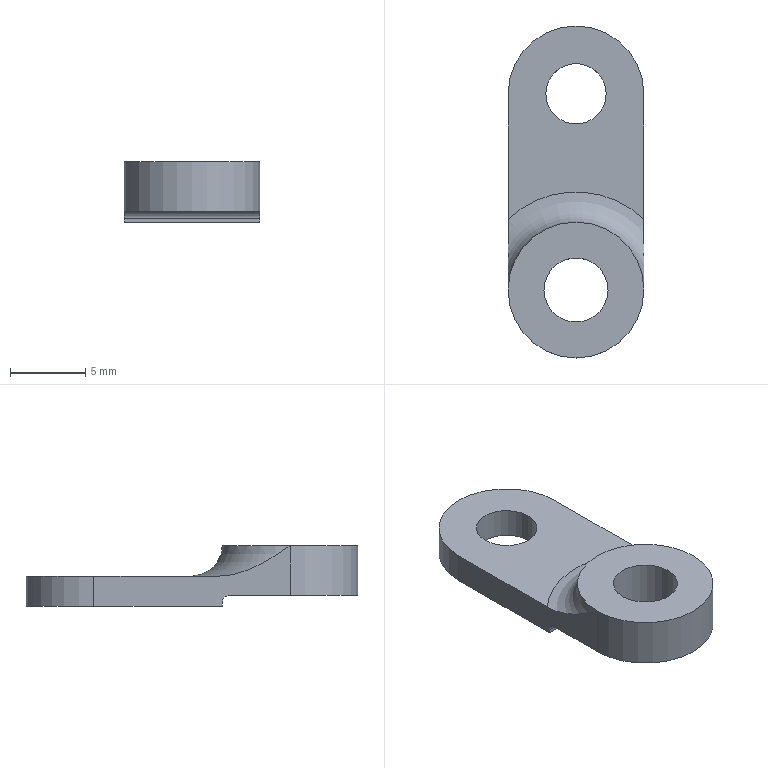Part | NX | 1 solid | 13 faces | box 9 x 22 x 4 mm | volume 375.215 mm3 | plane 7 | cylinder 5 | torus 1 | commonest cylinder face diameters 9 x2 1 x1 4 x1 4.25 x1
STEP:
#1=CARTESIAN_POINT('',(-4.5,-8.5,-1.78));
#2=VERTEX_POINT('',#1);
#3=CARTESIAN_POINT('',(-4.5,-8.5,-2.));
#4=VERTEX_POINT('',#3);
#5=CARTESIAN_POINT('',(-4.5,-8.5,-2.));
#6=DIRECTION('',(0.,0.,-1.));
#7=VECTOR('',#6,1000.);
#8=LINE('',#5,#7);
#9=EDGE_CURVE('',#2,#4,#8,.T.);
#10=ORIENTED_EDGE('',*,*,#9,.F.);
#11=CARTESIAN_POINT('',(-4.5,-9.,-1.28));
#12=VERTEX_POINT('',#11);
#13=CARTESIAN_POINT('',(-4.5,-9.,-1.78));
#14=DIRECTION('',(-1.,0.,0.));
#15=DIRECTION('',(0.,0.,1.));
#16=AXIS2_PLACEMENT_3D('',#13,#14,#15);
#17=CIRCLE('',#16,0.5);
#18=EDGE_CURVE('',#2,#12,#17,.F.);
#19=ORIENTED_EDGE('',*,*,#18,.T.);
#20=CARTESIAN_POINT('',(-4.5,-13.,-1.28));
#21=VERTEX_POINT('',#20);
#22=CARTESIAN_POINT('',(-4.5,0.,-1.28));
#23=DIRECTION('',(0.,1.,0.));
#24=VECTOR('',#23,1000.);
#25=LINE('',#22,#24);
#26=EDGE_CURVE('',#12,#21,#25,.F.);
#27=ORIENTED_EDGE('',*,*,#26,.T.);
#28=CARTESIAN_POINT('',(-4.5,-13.,2.));
#29=VERTEX_POINT('',#28);
#30=CARTESIAN_POINT('',(-4.5,-13.,-2.));
#31=DIRECTION('',(0.,0.,1.));
#32=VECTOR('',#31,1000.);
#33=LINE('',#30,#32);
#34=EDGE_CURVE('',#21,#29,#33,.T.);
#35=ORIENTED_EDGE('',*,*,#34,.T.);
#36=CARTESIAN_POINT('',(-4.5,-8.31,0.));
#37=VERTEX_POINT('',#36);
#38=CARTESIAN_POINT('',(-4.5,-8.31,0.));
#39=CARTESIAN_POINT('',(-4.5,-9.186,0.));
#40=CARTESIAN_POINT('',(-4.5,-10.86,0.5704));
#41=CARTESIAN_POINT('',(-4.5,-12.281,1.521));
#42=CARTESIAN_POINT('',(-4.5,-13.,2.));
#43=B_SPLINE_CURVE_WITH_KNOTS('',3,(#38,#39,#40,#41,#42),.UNSPECIFIED.,.F.,.F.,(4,1,4),(0.,0.002591,0.005182),.UNSPECIFIED.);
#44=EDGE_CURVE('',#29,#37,#43,.F.);
#45=ORIENTED_EDGE('',*,*,#44,.T.);
#46=CARTESIAN_POINT('',(-4.5,0.,0.));
#47=VERTEX_POINT('',#46);
#48=CARTESIAN_POINT('',(-4.5,0.,0.));
#49=DIRECTION('',(0.,-1.,0.));
#50=VECTOR('',#49,1000.);
#51=LINE('',#48,#50);
#52=EDGE_CURVE('',#47,#37,#51,.T.);
#53=ORIENTED_EDGE('',*,*,#52,.F.);
#54=CARTESIAN_POINT('',(-4.5,0.,-2.));
#55=VERTEX_POINT('',#54);
#56=CARTESIAN_POINT('',(-4.5,0.,-2.));
#57=DIRECTION('',(0.,0.,1.));
#58=VECTOR('',#57,1000.);
#59=LINE('',#56,#58);
#60=EDGE_CURVE('',#55,#47,#59,.T.);
#61=ORIENTED_EDGE('',*,*,#60,.F.);
#62=CARTESIAN_POINT('',(-4.5,0.,-2.));
#63=DIRECTION('',(0.,-1.,0.));
#64=VECTOR('',#63,1000.);
#65=LINE('',#62,#64);
#66=EDGE_CURVE('',#55,#4,#65,.T.);
#67=ORIENTED_EDGE('',*,*,#66,.T.);
#68=EDGE_LOOP('',(#10,#19,#27,#35,#45,#53,#61,#67));
#69=FACE_BOUND('',#68,.T.);
#70=CARTESIAN_POINT('',(-4.5,0.,-2.));
#71=DIRECTION('',(-1.,0.,0.));
#72=DIRECTION('',(0.,0.,1.));
#73=AXIS2_PLACEMENT_3D('',#70,#71,#72);
#74=PLANE('',#73);
#75=ADVANCED_FACE('',(#69),#74,.T.);
#76=ORIENTED_EDGE('',*,*,#60,.T.);
#77=CARTESIAN_POINT('',(4.5,0.,0.));
#78=VERTEX_POINT('',#77);
#79=CARTESIAN_POINT('',(0.,0.,0.));
#80=DIRECTION('',(0.,0.,1.));
#81=DIRECTION('',(1.,0.,0.));
#82=AXIS2_PLACEMENT_3D('',#79,#80,#81);
#83=CIRCLE('',#82,4.5);
#84=EDGE_CURVE('',#78,#47,#83,.T.);
#85=ORIENTED_EDGE('',*,*,#84,.F.);
#86=CARTESIAN_POINT('',(4.5,0.,-2.));
#87=VERTEX_POINT('',#86);
#88=CARTESIAN_POINT('',(4.5,0.,-2.));
#89=DIRECTION('',(0.,0.,1.));
#90=VECTOR('',#89,1000.);
#91=LINE('',#88,#90);
#92=EDGE_CURVE('',#87,#78,#91,.T.);
#93=ORIENTED_EDGE('',*,*,#92,.F.);
#94=CARTESIAN_POINT('',(0.,0.,-2.));
#95=DIRECTION('',(0.,0.,1.));
#96=DIRECTION('',(1.,0.,0.));
#97=AXIS2_PLACEMENT_3D('',#94,#95,#96);
#98=CIRCLE('',#97,4.5);
#99=EDGE_CURVE('',#87,#55,#98,.T.);
#100=ORIENTED_EDGE('',*,*,#99,.T.);
#101=EDGE_LOOP('',(#76,#85,#93,#100));
#102=FACE_BOUND('',#101,.T.);
#103=CARTESIAN_POINT('',(0.,0.,-2.));
#104=DIRECTION('',(0.,0.,1.));
#105=DIRECTION('',(1.,0.,0.));
#106=AXIS2_PLACEMENT_3D('',#103,#104,#105);
#107=CYLINDRICAL_SURFACE('',#106,4.5);
#108=ADVANCED_FACE('',(#102),#107,.T.);
#109=CARTESIAN_POINT('',(4.5,-13.,-1.28));
#110=VERTEX_POINT('',#109);
#111=CARTESIAN_POINT('',(4.5,-9.,-1.28));
#112=VERTEX_POINT('',#111);
#113=CARTESIAN_POINT('',(4.5,-13.,-1.28));
#114=DIRECTION('',(0.,-1.,0.));
#115=VECTOR('',#114,1000.);
#116=LINE('',#113,#115);
#117=EDGE_CURVE('',#110,#112,#116,.F.);
#118=ORIENTED_EDGE('',*,*,#117,.T.);
#119=CARTESIAN_POINT('',(4.5,-8.5,-1.78));
#120=VERTEX_POINT('',#119);
#121=CARTESIAN_POINT('',(4.5,-9.,-1.78));
#122=DIRECTION('',(1.,0.,0.));
#123=DIRECTION('',(0.,0.,-1.));
#124=AXIS2_PLACEMENT_3D('',#121,#122,#123);
#125=CIRCLE('',#124,0.5);
#126=EDGE_CURVE('',#112,#120,#125,.F.);
#127=ORIENTED_EDGE('',*,*,#126,.T.);
#128=CARTESIAN_POINT('',(4.5,-8.5,-2.));
#129=VERTEX_POINT('',#128);
#130=CARTESIAN_POINT('',(4.5,-8.5,-2.));
#131=DIRECTION('',(0.,0.,1.));
#132=VECTOR('',#131,1000.);
#133=LINE('',#130,#132);
#134=EDGE_CURVE('',#120,#129,#133,.F.);
#135=ORIENTED_EDGE('',*,*,#134,.T.);
#136=CARTESIAN_POINT('',(4.5,-13.,-2.));
#137=DIRECTION('',(0.,1.,0.));
#138=VECTOR('',#137,1000.);
#139=LINE('',#136,#138);
#140=EDGE_CURVE('',#129,#87,#139,.T.);
#141=ORIENTED_EDGE('',*,*,#140,.T.);
#142=ORIENTED_EDGE('',*,*,#92,.T.);
#143=CARTESIAN_POINT('',(4.5,-8.31,0.));
#144=VERTEX_POINT('',#143);
#145=CARTESIAN_POINT('',(4.5,-13.,0.));
#146=DIRECTION('',(0.,1.,0.));
#147=VECTOR('',#146,1000.);
#148=LINE('',#145,#147);
#149=EDGE_CURVE('',#144,#78,#148,.T.);
#150=ORIENTED_EDGE('',*,*,#149,.F.);
#151=CARTESIAN_POINT('',(4.5,-13.,2.));
#152=VERTEX_POINT('',#151);
#153=CARTESIAN_POINT('',(4.5,-8.31,0.));
#154=CARTESIAN_POINT('',(4.5,-9.186,0.));
#155=CARTESIAN_POINT('',(4.5,-10.86,0.5704));
#156=CARTESIAN_POINT('',(4.5,-12.281,1.521));
#157=CARTESIAN_POINT('',(4.5,-13.,2.));
#158=B_SPLINE_CURVE_WITH_KNOTS('',3,(#153,#154,#155,#156,#157),.UNSPECIFIED.,.F.,.F.,(4,1,4),(0.,0.002591,0.005182),.UNSPECIFIED.);
#159=EDGE_CURVE('',#144,#152,#158,.T.);
#160=ORIENTED_EDGE('',*,*,#159,.T.);
#161=CARTESIAN_POINT('',(4.5,-13.,-2.));
#162=DIRECTION('',(0.,0.,1.));
#163=VECTOR('',#162,1000.);
#164=LINE('',#161,#163);
#165=EDGE_CURVE('',#110,#152,#164,.T.);
#166=ORIENTED_EDGE('',*,*,#165,.F.);
#167=EDGE_LOOP('',(#118,#127,#135,#141,#142,#150,#160,#166));
#168=FACE_BOUND('',#167,.T.);
#169=CARTESIAN_POINT('',(4.5,-13.,-2.));
#170=DIRECTION('',(1.,0.,0.));
#171=DIRECTION('',(0.,0.,-1.));
#172=AXIS2_PLACEMENT_3D('',#169,#170,#171);
#173=PLANE('',#172);
#174=ADVANCED_FACE('',(#168),#173,.T.);
#175=CARTESIAN_POINT('',(2.,0.,-2.));
#176=VERTEX_POINT('',#175);
#177=CARTESIAN_POINT('',(0.,0.,-2.));
#178=DIRECTION('',(0.,0.,1.));
#179=DIRECTION('',(1.,0.,0.));
#180=AXIS2_PLACEMENT_3D('',#177,#178,#179);
#181=CIRCLE('',#180,2.);
#182=EDGE_CURVE('',#176,#176,#181,.F.);
#183=ORIENTED_EDGE('',*,*,#182,.F.);
#184=EDGE_LOOP('',(#183));
#185=FACE_BOUND('',#184,.T.);
#186=ORIENTED_EDGE('',*,*,#140,.F.);
#187=CARTESIAN_POINT('',(0.,-8.5,-2.));
#188=DIRECTION('',(-1.,0.,0.));
#189=VECTOR('',#188,1000.);
#190=LINE('',#187,#189);
#191=EDGE_CURVE('',#129,#4,#190,.T.);
#192=ORIENTED_EDGE('',*,*,#191,.T.);
#193=ORIENTED_EDGE('',*,*,#66,.F.);
#194=ORIENTED_EDGE('',*,*,#99,.F.);
#195=EDGE_LOOP('',(#186,#192,#193,#194));
#196=FACE_BOUND('',#195,.T.);
#197=CARTESIAN_POINT('',(0.,-13.,-2.));
#198=DIRECTION('',(0.,0.,1.));
#199=DIRECTION('',(1.,0.,0.));
#200=AXIS2_PLACEMENT_3D('',#197,#198,#199);
#201=PLANE('',#200);
#202=ADVANCED_FACE('',(#185,#196),#201,.F.);
#203=ORIENTED_EDGE('',*,*,#182,.T.);
#204=EDGE_LOOP('',(#203));
#205=FACE_BOUND('',#204,.T.);
#206=CARTESIAN_POINT('',(2.,0.,0.));
#207=VERTEX_POINT('',#206);
#208=CARTESIAN_POINT('',(0.,0.,0.));
#209=DIRECTION('',(0.,0.,-1.));
#210=DIRECTION('',(1.,0.,0.));
#211=AXIS2_PLACEMENT_3D('',#208,#209,#210);
#212=CIRCLE('',#211,2.);
#213=EDGE_CURVE('',#207,#207,#212,.T.);
#214=ORIENTED_EDGE('',*,*,#213,.F.);
#215=EDGE_LOOP('',(#214));
#216=FACE_BOUND('',#215,.T.);
#217=CARTESIAN_POINT('',(0.,0.,-25.));
#218=DIRECTION('',(0.,0.,1.));
#219=DIRECTION('',(1.,0.,0.));
#220=AXIS2_PLACEMENT_3D('',#217,#218,#219);
#221=CYLINDRICAL_SURFACE('',#220,2.);
#222=ADVANCED_FACE('',(#205,#216),#221,.F.);
#223=ORIENTED_EDGE('',*,*,#134,.F.);
#224=CARTESIAN_POINT('',(-4.5,-8.5,-1.78));
#225=DIRECTION('',(-1.,0.,0.));
#226=VECTOR('',#225,1000.);
#227=LINE('',#224,#226);
#228=EDGE_CURVE('',#120,#2,#227,.T.);
#229=ORIENTED_EDGE('',*,*,#228,.T.);
#230=ORIENTED_EDGE('',*,*,#9,.T.);
#231=ORIENTED_EDGE('',*,*,#191,.F.);
#232=EDGE_LOOP('',(#223,#229,#230,#231));
#233=FACE_BOUND('',#232,.T.);
#234=CARTESIAN_POINT('',(0.,-8.5,-2.));
#235=DIRECTION('',(0.,1.,0.));
#236=DIRECTION('',(0.,0.,1.));
#237=AXIS2_PLACEMENT_3D('',#234,#235,#236);
#238=PLANE('',#237);
#239=ADVANCED_FACE('',(#233),#238,.F.);
#240=ORIENTED_EDGE('',*,*,#213,.T.);
#241=EDGE_LOOP('',(#240));
#242=FACE_BOUND('',#241,.T.);
#243=ORIENTED_EDGE('',*,*,#52,.T.);
#244=CARTESIAN_POINT('',(0.,-13.,0.));
#245=DIRECTION('',(0.,0.,1.));
#246=DIRECTION('',(1.,0.,0.));
#247=AXIS2_PLACEMENT_3D('',#244,#245,#246);
#248=CIRCLE('',#247,6.5);
#249=EDGE_CURVE('',#37,#144,#248,.F.);
#250=ORIENTED_EDGE('',*,*,#249,.T.);
#251=ORIENTED_EDGE('',*,*,#149,.T.);
#252=ORIENTED_EDGE('',*,*,#84,.T.);
#253=EDGE_LOOP('',(#243,#250,#251,#252));
#254=FACE_BOUND('',#253,.T.);
#255=CARTESIAN_POINT('',(0.,-13.,0.));
#256=DIRECTION('',(0.,0.,1.));
#257=DIRECTION('',(1.,0.,0.));
#258=AXIS2_PLACEMENT_3D('',#255,#256,#257);
#259=PLANE('',#258);
#260=ADVANCED_FACE('',(#242,#254),#259,.T.);
#261=CARTESIAN_POINT('',(0.,-13.,-1.28));
#262=DIRECTION('',(0.,0.,1.));
#263=DIRECTION('',(1.,0.,0.));
#264=AXIS2_PLACEMENT_3D('',#261,#262,#263);
#265=CIRCLE('',#264,4.5);
#266=EDGE_CURVE('',#21,#110,#265,.T.);
#267=ORIENTED_EDGE('',*,*,#266,.T.);
#268=ORIENTED_EDGE('',*,*,#165,.T.);
#269=CARTESIAN_POINT('',(0.,-13.,2.));
#270=DIRECTION('',(0.,0.,-1.));
#271=DIRECTION('',(1.,0.,0.));
#272=AXIS2_PLACEMENT_3D('',#269,#270,#271);
#273=CIRCLE('',#272,4.5);
#274=EDGE_CURVE('',#152,#29,#273,.T.);
#275=ORIENTED_EDGE('',*,*,#274,.T.);
#276=ORIENTED_EDGE('',*,*,#34,.F.);
#277=EDGE_LOOP('',(#267,#268,#275,#276));
#278=FACE_BOUND('',#277,.T.);
#279=CARTESIAN_POINT('',(0.,-13.,-2.));
#280=DIRECTION('',(0.,0.,1.));
#281=DIRECTION('',(1.,0.,0.));
#282=AXIS2_PLACEMENT_3D('',#279,#280,#281);
#283=CYLINDRICAL_SURFACE('',#282,4.5);
#284=ADVANCED_FACE('',(#278),#283,.T.);
#285=CARTESIAN_POINT('',(2.125,-13.,-1.28));
#286=VERTEX_POINT('',#285);
#287=CARTESIAN_POINT('',(0.,-13.,-1.28));
#288=DIRECTION('',(0.,0.,1.));
#289=DIRECTION('',(1.,0.,0.));
#290=AXIS2_PLACEMENT_3D('',#287,#288,#289);
#291=CIRCLE('',#290,2.125);
#292=EDGE_CURVE('',#286,#286,#291,.F.);
#293=ORIENTED_EDGE('',*,*,#292,.T.);
#294=EDGE_LOOP('',(#293));
#295=FACE_BOUND('',#294,.T.);
#296=CARTESIAN_POINT('',(2.125,-13.,2.));
#297=VERTEX_POINT('',#296);
#298=CARTESIAN_POINT('',(0.,-13.,2.));
#299=DIRECTION('',(0.,0.,1.));
#300=DIRECTION('',(1.,0.,0.));
#301=AXIS2_PLACEMENT_3D('',#298,#299,#300);
#302=CIRCLE('',#301,2.125);
#303=EDGE_CURVE('',#297,#297,#302,.T.);
#304=ORIENTED_EDGE('',*,*,#303,.T.);
#305=EDGE_LOOP('',(#304));
#306=FACE_BOUND('',#305,.T.);
#307=CARTESIAN_POINT('',(0.,-13.,2.));
#308=DIRECTION('',(0.,0.,-1.));
#309=DIRECTION('',(-1.,0.,0.));
#310=AXIS2_PLACEMENT_3D('',#307,#308,#309);
#311=CYLINDRICAL_SURFACE('',#310,2.125);
#312=ADVANCED_FACE('',(#295,#306),#311,.F.);
#313=ORIENTED_EDGE('',*,*,#274,.F.);
#314=CARTESIAN_POINT('',(0.,-13.,2.));
#315=DIRECTION('',(0.,0.,-1.));
#316=DIRECTION('',(1.,0.,0.));
#317=AXIS2_PLACEMENT_3D('',#314,#315,#316);
#318=CIRCLE('',#317,4.5);
#319=EDGE_CURVE('',#29,#152,#318,.T.);
#320=ORIENTED_EDGE('',*,*,#319,.F.);
#321=EDGE_LOOP('',(#313,#320));
#322=FACE_BOUND('',#321,.T.);
#323=ORIENTED_EDGE('',*,*,#303,.F.);
#324=EDGE_LOOP('',(#323));
#325=FACE_BOUND('',#324,.T.);
#326=CARTESIAN_POINT('',(0.,-13.,2.));
#327=DIRECTION('',(0.,0.,-1.));
#328=DIRECTION('',(-1.,0.,0.));
#329=AXIS2_PLACEMENT_3D('',#326,#327,#328);
#330=PLANE('',#329);
#331=ADVANCED_FACE('',(#322,#325),#330,.F.);
#332=ORIENTED_EDGE('',*,*,#44,.F.);
#333=ORIENTED_EDGE('',*,*,#319,.T.);
#334=ORIENTED_EDGE('',*,*,#159,.F.);
#335=ORIENTED_EDGE('',*,*,#249,.F.);
#336=EDGE_LOOP('',(#332,#333,#334,#335));
#337=FACE_BOUND('',#336,.T.);
#338=CARTESIAN_POINT('',(0.,-13.,2.));
#339=DIRECTION('',(0.,0.,1.));
#340=DIRECTION('',(1.,0.,0.));
#341=AXIS2_PLACEMENT_3D('',#338,#339,#340);
#342=TOROIDAL_SURFACE('',#341,6.5,2.);
#343=ADVANCED_FACE('',(#337),#342,.F.);
#344=ORIENTED_EDGE('',*,*,#26,.F.);
#345=CARTESIAN_POINT('',(4.5,-9.,-1.28));
#346=DIRECTION('',(-1.,0.,0.));
#347=VECTOR('',#346,1000.);
#348=LINE('',#345,#347);
#349=EDGE_CURVE('',#12,#112,#348,.F.);
#350=ORIENTED_EDGE('',*,*,#349,.T.);
#351=ORIENTED_EDGE('',*,*,#117,.F.);
#352=ORIENTED_EDGE('',*,*,#266,.F.);
#353=EDGE_LOOP('',(#344,#350,#351,#352));
#354=FACE_BOUND('',#353,.T.);
#355=ORIENTED_EDGE('',*,*,#292,.F.);
#356=EDGE_LOOP('',(#355));
#357=FACE_BOUND('',#356,.T.);
#358=CARTESIAN_POINT('',(0.,-13.,-1.28));
#359=DIRECTION('',(0.,0.,1.));
#360=DIRECTION('',(1.,0.,0.));
#361=AXIS2_PLACEMENT_3D('',#358,#359,#360);
#362=PLANE('',#361);
#363=ADVANCED_FACE('',(#354,#357),#362,.F.);
#364=ORIENTED_EDGE('',*,*,#126,.F.);
#365=ORIENTED_EDGE('',*,*,#349,.F.);
#366=ORIENTED_EDGE('',*,*,#18,.F.);
#367=ORIENTED_EDGE('',*,*,#228,.F.);
#368=EDGE_LOOP('',(#364,#365,#366,#367));
#369=FACE_BOUND('',#368,.T.);
#370=CARTESIAN_POINT('',(0.,-9.,-1.78));
#371=DIRECTION('',(1.,0.,0.));
#372=DIRECTION('',(0.,0.,-1.));
#373=AXIS2_PLACEMENT_3D('',#370,#371,#372);
#374=CYLINDRICAL_SURFACE('',#373,0.5);
#375=ADVANCED_FACE('',(#369),#374,.F.);
#376=CLOSED_SHELL('',(#75,#108,#174,#202,#222,#239,#260,#284,#312,#331,#343,#363,#375));
#377=MANIFOLD_SOLID_BREP('',#376);
#378=(LENGTH_UNIT()NAMED_UNIT(*)SI_UNIT(.MILLI.,.METRE.));
#379=UNCERTAINTY_MEASURE_WITH_UNIT(LENGTH_MEASURE(0.0508),#378,'','');
#380=(NAMED_UNIT(*)PLANE_ANGLE_UNIT()SI_UNIT($,.RADIAN.));
#381=(NAMED_UNIT(*)SI_UNIT($,.STERADIAN.)SOLID_ANGLE_UNIT());
#382=(GEOMETRIC_REPRESENTATION_CONTEXT(3)GLOBAL_UNCERTAINTY_ASSIGNED_CONTEXT((#379))GLOBAL_UNIT_ASSIGNED_CONTEXT((#378,#380,#381))REPRESENTATION_CONTEXT('',''));
#383=ADVANCED_BREP_SHAPE_REPRESENTATION('',(#377),#382);